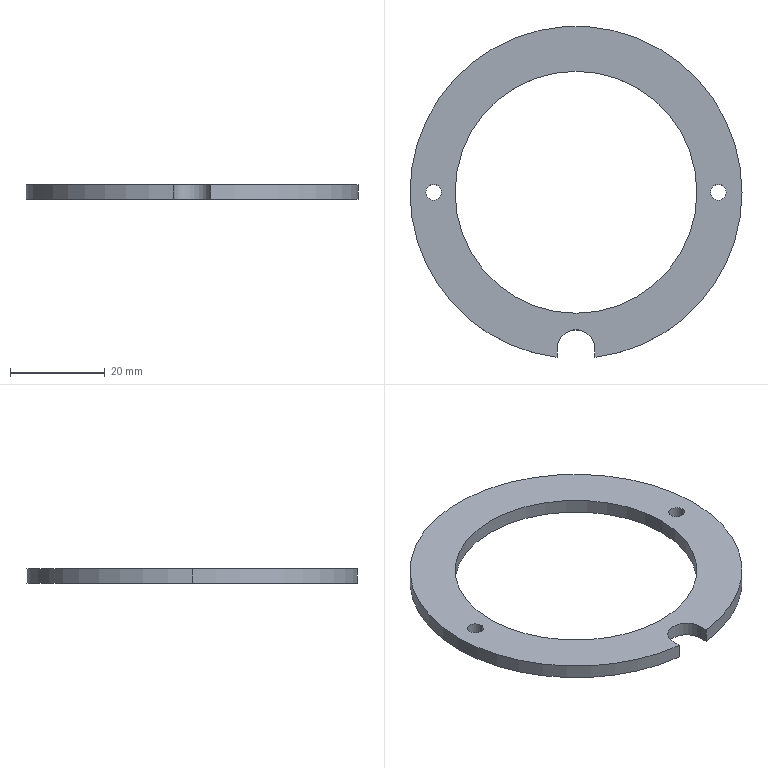Part | SolidWorks | features ICE 4, Extrusion 1, HoleWzd 1 | 1 solid | 14 faces | box 70 x 69.771 x 3 mm | volume 5244 mm3 | cylinder 10 | plane 4 | commonest cylinder face diameters 3.3 x4 70 x3 51 x2 8 x1
STEP:
#1=CARTESIAN_POINT('',(28.35,0.,0.));
#2=VERTEX_POINT('',#1);
#3=CARTESIAN_POINT('',(31.65,0.,0.));
#4=VERTEX_POINT('',#3);
#5=CARTESIAN_POINT('',(30.,0.,0.));
#6=DIRECTION('',(0.,0.,1.));
#7=DIRECTION('',(1.,0.,0.));
#8=AXIS2_PLACEMENT_3D('',#5,#6,#7);
#9=CIRCLE('',#8,1.65);
#10=EDGE_CURVE('',#2,#4,#9,.T.);
#11=ORIENTED_EDGE('',*,*,#10,.F.);
#12=CARTESIAN_POINT('',(28.35,0.,3.));
#13=VERTEX_POINT('',#12);
#14=CARTESIAN_POINT('',(28.35,0.,0.));
#15=DIRECTION('',(0.,0.,1.));
#16=VECTOR('',#15,1000.);
#17=LINE('',#14,#16);
#18=EDGE_CURVE('',#2,#13,#17,.T.);
#19=ORIENTED_EDGE('',*,*,#18,.T.);
#20=CARTESIAN_POINT('',(31.65,0.,3.));
#21=VERTEX_POINT('',#20);
#22=CARTESIAN_POINT('',(30.,0.,3.));
#23=DIRECTION('',(0.,0.,1.));
#24=DIRECTION('',(1.,0.,0.));
#25=AXIS2_PLACEMENT_3D('',#22,#23,#24);
#26=CIRCLE('',#25,1.65);
#27=EDGE_CURVE('',#13,#21,#26,.T.);
#28=ORIENTED_EDGE('',*,*,#27,.T.);
#29=CARTESIAN_POINT('',(31.65,0.,0.));
#30=DIRECTION('',(0.,0.,1.));
#31=VECTOR('',#30,1000.);
#32=LINE('',#29,#31);
#33=EDGE_CURVE('',#4,#21,#32,.T.);
#34=ORIENTED_EDGE('',*,*,#33,.F.);
#35=EDGE_LOOP('',(#11,#19,#28,#34));
#36=FACE_OUTER_BOUND('',#35,.T.);
#37=CARTESIAN_POINT('',(30.,0.,0.));
#38=DIRECTION('',(0.,0.,1.));
#39=DIRECTION('',(1.,0.,0.));
#40=AXIS2_PLACEMENT_3D('',#37,#38,#39);
#41=CYLINDRICAL_SURFACE('',#40,1.65);
#42=ADVANCED_FACE('',(#36),#41,.F.);
#43=CARTESIAN_POINT('',(-31.65,0.,0.));
#44=VERTEX_POINT('',#43);
#45=CARTESIAN_POINT('',(-28.35,0.,0.));
#46=VERTEX_POINT('',#45);
#47=CARTESIAN_POINT('',(-30.,0.,0.));
#48=DIRECTION('',(0.,0.,1.));
#49=DIRECTION('',(-1.,0.,0.));
#50=AXIS2_PLACEMENT_3D('',#47,#48,#49);
#51=CIRCLE('',#50,1.65);
#52=EDGE_CURVE('',#44,#46,#51,.T.);
#53=ORIENTED_EDGE('',*,*,#52,.F.);
#54=CARTESIAN_POINT('',(-31.65,0.,3.));
#55=VERTEX_POINT('',#54);
#56=CARTESIAN_POINT('',(-31.65,0.,0.));
#57=DIRECTION('',(0.,0.,1.));
#58=VECTOR('',#57,1000.);
#59=LINE('',#56,#58);
#60=EDGE_CURVE('',#44,#55,#59,.T.);
#61=ORIENTED_EDGE('',*,*,#60,.T.);
#62=CARTESIAN_POINT('',(-28.35,0.,3.));
#63=VERTEX_POINT('',#62);
#64=CARTESIAN_POINT('',(-30.,0.,3.));
#65=DIRECTION('',(0.,0.,1.));
#66=DIRECTION('',(-1.,0.,0.));
#67=AXIS2_PLACEMENT_3D('',#64,#65,#66);
#68=CIRCLE('',#67,1.65);
#69=EDGE_CURVE('',#55,#63,#68,.T.);
#70=ORIENTED_EDGE('',*,*,#69,.T.);
#71=CARTESIAN_POINT('',(-28.35,0.,0.));
#72=DIRECTION('',(0.,0.,1.));
#73=VECTOR('',#72,1000.);
#74=LINE('',#71,#73);
#75=EDGE_CURVE('',#46,#63,#74,.T.);
#76=ORIENTED_EDGE('',*,*,#75,.F.);
#77=EDGE_LOOP('',(#53,#61,#70,#76));
#78=FACE_OUTER_BOUND('',#77,.T.);
#79=CARTESIAN_POINT('',(-30.,0.,0.));
#80=DIRECTION('',(0.,0.,1.));
#81=DIRECTION('',(1.,0.,0.));
#82=AXIS2_PLACEMENT_3D('',#79,#80,#81);
#83=CYLINDRICAL_SURFACE('',#82,1.65);
#84=ADVANCED_FACE('',(#78),#83,.F.);
#85=CARTESIAN_POINT('',(-25.5,0.,3.));
#86=VERTEX_POINT('',#85);
#87=CARTESIAN_POINT('',(25.5,0.,3.));
#88=VERTEX_POINT('',#87);
#89=CARTESIAN_POINT('',(0.,0.,3.));
#90=DIRECTION('',(0.,0.,1.));
#91=DIRECTION('',(1.,0.,0.));
#92=AXIS2_PLACEMENT_3D('',#89,#90,#91);
#93=CIRCLE('',#92,25.5);
#94=EDGE_CURVE('',#86,#88,#93,.T.);
#95=ORIENTED_EDGE('',*,*,#94,.T.);
#96=CARTESIAN_POINT('',(25.5,0.,0.));
#97=VERTEX_POINT('',#96);
#98=CARTESIAN_POINT('',(25.5,0.,3.));
#99=DIRECTION('',(0.,0.,-1.));
#100=VECTOR('',#99,1000.);
#101=LINE('',#98,#100);
#102=EDGE_CURVE('',#88,#97,#101,.T.);
#103=ORIENTED_EDGE('',*,*,#102,.T.);
#104=CARTESIAN_POINT('',(-25.5,0.,0.));
#105=VERTEX_POINT('',#104);
#106=CARTESIAN_POINT('',(0.,0.,0.));
#107=DIRECTION('',(0.,0.,1.));
#108=DIRECTION('',(1.,0.,0.));
#109=AXIS2_PLACEMENT_3D('',#106,#107,#108);
#110=CIRCLE('',#109,25.5);
#111=EDGE_CURVE('',#105,#97,#110,.T.);
#112=ORIENTED_EDGE('',*,*,#111,.F.);
#113=CARTESIAN_POINT('',(-25.5,0.,3.));
#114=DIRECTION('',(0.,0.,-1.));
#115=VECTOR('',#114,1000.);
#116=LINE('',#113,#115);
#117=EDGE_CURVE('',#86,#105,#116,.T.);
#118=ORIENTED_EDGE('',*,*,#117,.F.);
#119=EDGE_LOOP('',(#95,#103,#112,#118));
#120=FACE_OUTER_BOUND('',#119,.T.);
#121=CARTESIAN_POINT('',(0.,0.,3.));
#122=DIRECTION('',(0.,0.,-1.));
#123=DIRECTION('',(-1.,0.,0.));
#124=AXIS2_PLACEMENT_3D('',#121,#122,#123);
#125=CYLINDRICAL_SURFACE('',#124,25.5);
#126=ADVANCED_FACE('',(#120),#125,.F.);
#127=CARTESIAN_POINT('',(35.,0.,3.));
#128=VERTEX_POINT('',#127);
#129=CARTESIAN_POINT('',(-35.,0.,3.));
#130=VERTEX_POINT('',#129);
#131=CARTESIAN_POINT('',(0.,0.,3.));
#132=DIRECTION('',(0.,0.,1.));
#133=DIRECTION('',(1.,0.,0.));
#134=AXIS2_PLACEMENT_3D('',#131,#132,#133);
#135=CIRCLE('',#134,35.);
#136=EDGE_CURVE('',#128,#130,#135,.T.);
#137=ORIENTED_EDGE('',*,*,#136,.F.);
#138=CARTESIAN_POINT('',(35.,0.,0.));
#139=VERTEX_POINT('',#138);
#140=CARTESIAN_POINT('',(35.,0.,3.));
#141=DIRECTION('',(0.,0.,-1.));
#142=VECTOR('',#141,1000.);
#143=LINE('',#140,#142);
#144=EDGE_CURVE('',#128,#139,#143,.T.);
#145=ORIENTED_EDGE('',*,*,#144,.T.);
#146=CARTESIAN_POINT('',(-35.,0.,0.));
#147=VERTEX_POINT('',#146);
#148=CARTESIAN_POINT('',(0.,0.,0.));
#149=DIRECTION('',(0.,0.,1.));
#150=DIRECTION('',(1.,0.,0.));
#151=AXIS2_PLACEMENT_3D('',#148,#149,#150);
#152=CIRCLE('',#151,35.);
#153=EDGE_CURVE('',#139,#147,#152,.T.);
#154=ORIENTED_EDGE('',*,*,#153,.T.);
#155=CARTESIAN_POINT('',(-35.,0.,3.));
#156=DIRECTION('',(0.,0.,-1.));
#157=VECTOR('',#156,1000.);
#158=LINE('',#155,#157);
#159=EDGE_CURVE('',#130,#147,#158,.T.);
#160=ORIENTED_EDGE('',*,*,#159,.F.);
#161=EDGE_LOOP('',(#137,#145,#154,#160));
#162=FACE_OUTER_BOUND('',#161,.T.);
#163=CARTESIAN_POINT('',(0.,0.,3.));
#164=DIRECTION('',(0.,0.,-1.));
#165=DIRECTION('',(-1.,0.,0.));
#166=AXIS2_PLACEMENT_3D('',#163,#164,#165);
#167=CYLINDRICAL_SURFACE('',#166,35.);
#168=ADVANCED_FACE('',(#162),#167,.T.);
#169=CARTESIAN_POINT('',(-4.,-34.771,3.));
#170=VERTEX_POINT('',#169);
#171=CARTESIAN_POINT('',(0.,0.,3.));
#172=DIRECTION('',(0.,0.,1.));
#173=DIRECTION('',(1.,0.,0.));
#174=AXIS2_PLACEMENT_3D('',#171,#172,#173);
#175=CIRCLE('',#174,35.);
#176=EDGE_CURVE('',#130,#170,#175,.T.);
#177=ORIENTED_EDGE('',*,*,#176,.F.);
#178=ORIENTED_EDGE('',*,*,#159,.T.);
#179=CARTESIAN_POINT('',(-4.,-34.771,0.));
#180=VERTEX_POINT('',#179);
#181=CARTESIAN_POINT('',(0.,0.,0.));
#182=DIRECTION('',(0.,0.,1.));
#183=DIRECTION('',(1.,0.,0.));
#184=AXIS2_PLACEMENT_3D('',#181,#182,#183);
#185=CIRCLE('',#184,35.);
#186=EDGE_CURVE('',#147,#180,#185,.T.);
#187=ORIENTED_EDGE('',*,*,#186,.T.);
#188=CARTESIAN_POINT('',(-4.,-34.771,3.));
#189=DIRECTION('',(0.,0.,1.));
#190=VECTOR('',#189,1000.);
#191=LINE('',#188,#190);
#192=EDGE_CURVE('',#180,#170,#191,.T.);
#193=ORIENTED_EDGE('',*,*,#192,.T.);
#194=EDGE_LOOP('',(#177,#178,#187,#193));
#195=FACE_OUTER_BOUND('',#194,.T.);
#196=CARTESIAN_POINT('',(0.,0.,3.));
#197=DIRECTION('',(0.,0.,-1.));
#198=DIRECTION('',(-1.,0.,0.));
#199=AXIS2_PLACEMENT_3D('',#196,#197,#198);
#200=CYLINDRICAL_SURFACE('',#199,35.);
#201=ADVANCED_FACE('',(#195),#200,.T.);
#202=CARTESIAN_POINT('',(30.,0.,3.));
#203=DIRECTION('',(0.,0.,1.));
#204=DIRECTION('',(1.,0.,0.));
#205=AXIS2_PLACEMENT_3D('',#202,#203,#204);
#206=CIRCLE('',#205,1.65);
#207=EDGE_CURVE('',#21,#13,#206,.T.);
#208=ORIENTED_EDGE('',*,*,#207,.F.);
#209=ORIENTED_EDGE('',*,*,#27,.F.);
#210=EDGE_LOOP('',(#208,#209));
#211=FACE_BOUND('',#210,.T.);
#212=CARTESIAN_POINT('',(-30.,0.,3.));
#213=DIRECTION('',(0.,0.,1.));
#214=DIRECTION('',(-1.,0.,0.));
#215=AXIS2_PLACEMENT_3D('',#212,#213,#214);
#216=CIRCLE('',#215,1.65);
#217=EDGE_CURVE('',#63,#55,#216,.T.);
#218=ORIENTED_EDGE('',*,*,#217,.F.);
#219=ORIENTED_EDGE('',*,*,#69,.F.);
#220=EDGE_LOOP('',(#218,#219));
#221=FACE_BOUND('',#220,.T.);
#222=CARTESIAN_POINT('',(4.,-34.771,3.));
#223=VERTEX_POINT('',#222);
#224=CARTESIAN_POINT('',(4.,-33.,3.));
#225=VERTEX_POINT('',#224);
#226=CARTESIAN_POINT('',(4.,-33.,3.));
#227=DIRECTION('',(0.,1.,0.));
#228=VECTOR('',#227,1000.);
#229=LINE('',#226,#228);
#230=EDGE_CURVE('',#223,#225,#229,.T.);
#231=ORIENTED_EDGE('',*,*,#230,.F.);
#232=CARTESIAN_POINT('',(0.,0.,3.));
#233=DIRECTION('',(0.,0.,1.));
#234=DIRECTION('',(1.,0.,0.));
#235=AXIS2_PLACEMENT_3D('',#232,#233,#234);
#236=CIRCLE('',#235,35.);
#237=EDGE_CURVE('',#223,#128,#236,.T.);
#238=ORIENTED_EDGE('',*,*,#237,.T.);
#239=ORIENTED_EDGE('',*,*,#136,.T.);
#240=ORIENTED_EDGE('',*,*,#176,.T.);
#241=CARTESIAN_POINT('',(-4.,-33.,3.));
#242=VERTEX_POINT('',#241);
#243=CARTESIAN_POINT('',(-4.,-33.,3.));
#244=DIRECTION('',(0.,-1.,0.));
#245=VECTOR('',#244,1000.);
#246=LINE('',#243,#245);
#247=EDGE_CURVE('',#242,#170,#246,.T.);
#248=ORIENTED_EDGE('',*,*,#247,.F.);
#249=CARTESIAN_POINT('',(0.,-33.,3.));
#250=DIRECTION('',(0.,0.,1.));
#251=DIRECTION('',(1.,0.,0.));
#252=AXIS2_PLACEMENT_3D('',#249,#250,#251);
#253=CIRCLE('',#252,4.);
#254=EDGE_CURVE('',#225,#242,#253,.T.);
#255=ORIENTED_EDGE('',*,*,#254,.F.);
#256=EDGE_LOOP('',(#231,#238,#239,#240,#248,#255));
#257=FACE_OUTER_BOUND('',#256,.T.);
#258=ORIENTED_EDGE('',*,*,#94,.F.);
#259=CARTESIAN_POINT('',(0.,0.,3.));
#260=DIRECTION('',(0.,0.,1.));
#261=DIRECTION('',(1.,0.,0.));
#262=AXIS2_PLACEMENT_3D('',#259,#260,#261);
#263=CIRCLE('',#262,25.5);
#264=EDGE_CURVE('',#88,#86,#263,.T.);
#265=ORIENTED_EDGE('',*,*,#264,.F.);
#266=EDGE_LOOP('',(#258,#265));
#267=FACE_BOUND('',#266,.T.);
#268=CARTESIAN_POINT('',(0.,0.,3.));
#269=DIRECTION('',(0.,0.,1.));
#270=DIRECTION('',(1.,0.,0.));
#271=AXIS2_PLACEMENT_3D('',#268,#269,#270);
#272=PLANE('',#271);
#273=ADVANCED_FACE('',(#211,#221,#257,#267),#272,.T.);
#274=CARTESIAN_POINT('',(30.,0.,0.));
#275=DIRECTION('',(0.,0.,1.));
#276=DIRECTION('',(1.,0.,0.));
#277=AXIS2_PLACEMENT_3D('',#274,#275,#276);
#278=CIRCLE('',#277,1.65);
#279=EDGE_CURVE('',#4,#2,#278,.T.);
#280=ORIENTED_EDGE('',*,*,#279,.T.);
#281=ORIENTED_EDGE('',*,*,#10,.T.);
#282=EDGE_LOOP('',(#280,#281));
#283=FACE_BOUND('',#282,.T.);
#284=CARTESIAN_POINT('',(-30.,0.,0.));
#285=DIRECTION('',(0.,0.,1.));
#286=DIRECTION('',(-1.,0.,0.));
#287=AXIS2_PLACEMENT_3D('',#284,#285,#286);
#288=CIRCLE('',#287,1.65);
#289=EDGE_CURVE('',#46,#44,#288,.T.);
#290=ORIENTED_EDGE('',*,*,#289,.T.);
#291=ORIENTED_EDGE('',*,*,#52,.T.);
#292=EDGE_LOOP('',(#290,#291));
#293=FACE_BOUND('',#292,.T.);
#294=CARTESIAN_POINT('',(4.,-34.771,0.));
#295=VERTEX_POINT('',#294);
#296=CARTESIAN_POINT('',(0.,0.,0.));
#297=DIRECTION('',(0.,0.,1.));
#298=DIRECTION('',(1.,0.,0.));
#299=AXIS2_PLACEMENT_3D('',#296,#297,#298);
#300=CIRCLE('',#299,35.);
#301=EDGE_CURVE('',#295,#139,#300,.T.);
#302=ORIENTED_EDGE('',*,*,#301,.F.);
#303=CARTESIAN_POINT('',(4.,-33.,0.));
#304=VERTEX_POINT('',#303);
#305=CARTESIAN_POINT('',(4.,-33.,0.));
#306=DIRECTION('',(0.,1.,0.));
#307=VECTOR('',#306,1000.);
#308=LINE('',#305,#307);
#309=EDGE_CURVE('',#295,#304,#308,.T.);
#310=ORIENTED_EDGE('',*,*,#309,.T.);
#311=CARTESIAN_POINT('',(-4.,-33.,0.));
#312=VERTEX_POINT('',#311);
#313=CARTESIAN_POINT('',(0.,-33.,0.));
#314=DIRECTION('',(0.,0.,-1.));
#315=DIRECTION('',(-1.,0.,0.));
#316=AXIS2_PLACEMENT_3D('',#313,#314,#315);
#317=CIRCLE('',#316,4.);
#318=EDGE_CURVE('',#312,#304,#317,.T.);
#319=ORIENTED_EDGE('',*,*,#318,.F.);
#320=CARTESIAN_POINT('',(-4.,-33.,0.));
#321=DIRECTION('',(0.,-1.,0.));
#322=VECTOR('',#321,1000.);
#323=LINE('',#320,#322);
#324=EDGE_CURVE('',#312,#180,#323,.T.);
#325=ORIENTED_EDGE('',*,*,#324,.T.);
#326=ORIENTED_EDGE('',*,*,#186,.F.);
#327=ORIENTED_EDGE('',*,*,#153,.F.);
#328=EDGE_LOOP('',(#302,#310,#319,#325,#326,#327));
#329=FACE_OUTER_BOUND('',#328,.T.);
#330=ORIENTED_EDGE('',*,*,#111,.T.);
#331=CARTESIAN_POINT('',(0.,0.,0.));
#332=DIRECTION('',(0.,0.,1.));
#333=DIRECTION('',(1.,0.,0.));
#334=AXIS2_PLACEMENT_3D('',#331,#332,#333);
#335=CIRCLE('',#334,25.5);
#336=EDGE_CURVE('',#97,#105,#335,.T.);
#337=ORIENTED_EDGE('',*,*,#336,.T.);
#338=EDGE_LOOP('',(#330,#337));
#339=FACE_BOUND('',#338,.T.);
#340=CARTESIAN_POINT('',(0.,0.,0.));
#341=DIRECTION('',(0.,0.,1.));
#342=DIRECTION('',(1.,0.,0.));
#343=AXIS2_PLACEMENT_3D('',#340,#341,#342);
#344=PLANE('',#343);
#345=ADVANCED_FACE('',(#283,#293,#329,#339),#344,.F.);
#346=ORIENTED_EDGE('',*,*,#144,.F.);
#347=ORIENTED_EDGE('',*,*,#237,.F.);
#348=CARTESIAN_POINT('',(4.,-34.771,3.));
#349=DIRECTION('',(0.,0.,-1.));
#350=VECTOR('',#349,1000.);
#351=LINE('',#348,#350);
#352=EDGE_CURVE('',#223,#295,#351,.T.);
#353=ORIENTED_EDGE('',*,*,#352,.T.);
#354=ORIENTED_EDGE('',*,*,#301,.T.);
#355=EDGE_LOOP('',(#346,#347,#353,#354));
#356=FACE_OUTER_BOUND('',#355,.T.);
#357=CARTESIAN_POINT('',(0.,0.,3.));
#358=DIRECTION('',(0.,0.,-1.));
#359=DIRECTION('',(-1.,0.,0.));
#360=AXIS2_PLACEMENT_3D('',#357,#358,#359);
#361=CYLINDRICAL_SURFACE('',#360,35.);
#362=ADVANCED_FACE('',(#356),#361,.T.);
#363=ORIENTED_EDGE('',*,*,#102,.F.);
#364=ORIENTED_EDGE('',*,*,#264,.T.);
#365=ORIENTED_EDGE('',*,*,#117,.T.);
#366=ORIENTED_EDGE('',*,*,#336,.F.);
#367=EDGE_LOOP('',(#363,#364,#365,#366));
#368=FACE_OUTER_BOUND('',#367,.T.);
#369=CARTESIAN_POINT('',(0.,0.,3.));
#370=DIRECTION('',(0.,0.,-1.));
#371=DIRECTION('',(-1.,0.,0.));
#372=AXIS2_PLACEMENT_3D('',#369,#370,#371);
#373=CYLINDRICAL_SURFACE('',#372,25.5);
#374=ADVANCED_FACE('',(#368),#373,.F.);
#375=ORIENTED_EDGE('',*,*,#318,.T.);
#376=CARTESIAN_POINT('',(4.,-33.,0.));
#377=DIRECTION('',(0.,0.,1.));
#378=VECTOR('',#377,1000.);
#379=LINE('',#376,#378);
#380=EDGE_CURVE('',#304,#225,#379,.T.);
#381=ORIENTED_EDGE('',*,*,#380,.T.);
#382=ORIENTED_EDGE('',*,*,#254,.T.);
#383=CARTESIAN_POINT('',(-4.,-33.,0.));
#384=DIRECTION('',(0.,0.,1.));
#385=VECTOR('',#384,1000.);
#386=LINE('',#383,#385);
#387=EDGE_CURVE('',#312,#242,#386,.T.);
#388=ORIENTED_EDGE('',*,*,#387,.F.);
#389=EDGE_LOOP('',(#375,#381,#382,#388));
#390=FACE_OUTER_BOUND('',#389,.T.);
#391=CARTESIAN_POINT('',(0.,-33.,5.));
#392=DIRECTION('',(0.,0.,-1.));
#393=DIRECTION('',(-1.,0.,0.));
#394=AXIS2_PLACEMENT_3D('',#391,#392,#393);
#395=CYLINDRICAL_SURFACE('',#394,4.);
#396=ADVANCED_FACE('',(#390),#395,.F.);
#397=ORIENTED_EDGE('',*,*,#324,.F.);
#398=ORIENTED_EDGE('',*,*,#387,.T.);
#399=ORIENTED_EDGE('',*,*,#247,.T.);
#400=ORIENTED_EDGE('',*,*,#192,.F.);
#401=EDGE_LOOP('',(#397,#398,#399,#400));
#402=FACE_OUTER_BOUND('',#401,.T.);
#403=CARTESIAN_POINT('',(-4.,-33.,0.));
#404=DIRECTION('',(-1.,0.,0.));
#405=DIRECTION('',(0.,-1.,0.));
#406=AXIS2_PLACEMENT_3D('',#403,#404,#405);
#407=PLANE('',#406);
#408=ADVANCED_FACE('',(#402),#407,.F.);
#409=ORIENTED_EDGE('',*,*,#230,.T.);
#410=ORIENTED_EDGE('',*,*,#380,.F.);
#411=ORIENTED_EDGE('',*,*,#309,.F.);
#412=ORIENTED_EDGE('',*,*,#352,.F.);
#413=EDGE_LOOP('',(#409,#410,#411,#412));
#414=FACE_OUTER_BOUND('',#413,.T.);
#415=CARTESIAN_POINT('',(4.,-33.,0.));
#416=DIRECTION('',(1.,0.,0.));
#417=DIRECTION('',(0.,1.,0.));
#418=AXIS2_PLACEMENT_3D('',#415,#416,#417);
#419=PLANE('',#418);
#420=ADVANCED_FACE('',(#414),#419,.F.);
#421=ORIENTED_EDGE('',*,*,#60,.F.);
#422=ORIENTED_EDGE('',*,*,#289,.F.);
#423=ORIENTED_EDGE('',*,*,#75,.T.);
#424=ORIENTED_EDGE('',*,*,#217,.T.);
#425=EDGE_LOOP('',(#421,#422,#423,#424));
#426=FACE_OUTER_BOUND('',#425,.T.);
#427=CARTESIAN_POINT('',(-30.,0.,0.));
#428=DIRECTION('',(0.,0.,1.));
#429=DIRECTION('',(1.,0.,0.));
#430=AXIS2_PLACEMENT_3D('',#427,#428,#429);
#431=CYLINDRICAL_SURFACE('',#430,1.65);
#432=ADVANCED_FACE('',(#426),#431,.F.);
#433=ORIENTED_EDGE('',*,*,#18,.F.);
#434=ORIENTED_EDGE('',*,*,#279,.F.);
#435=ORIENTED_EDGE('',*,*,#33,.T.);
#436=ORIENTED_EDGE('',*,*,#207,.T.);
#437=EDGE_LOOP('',(#433,#434,#435,#436));
#438=FACE_OUTER_BOUND('',#437,.T.);
#439=CARTESIAN_POINT('',(30.,0.,0.));
#440=DIRECTION('',(0.,0.,1.));
#441=DIRECTION('',(1.,0.,0.));
#442=AXIS2_PLACEMENT_3D('',#439,#440,#441);
#443=CYLINDRICAL_SURFACE('',#442,1.65);
#444=ADVANCED_FACE('',(#438),#443,.F.);
#445=CLOSED_SHELL('',(#42,#84,#126,#168,#201,#273,#345,#362,#374,#396,#408,#420,#432,#444));
#446=MANIFOLD_SOLID_BREP('',#445);
#447=CARTESIAN_POINT('',(0.,0.,0.));
#448=DIRECTION('',(0.,0.,1.));
#449=DIRECTION('',(1.,0.,0.));
#450=AXIS2_PLACEMENT_3D('',#447,#448,#449);
#451=(LENGTH_UNIT()NAMED_UNIT(*)SI_UNIT(.MILLI.,.METRE.));
#452=UNCERTAINTY_MEASURE_WITH_UNIT(LENGTH_MEASURE(0.00001),#451,'','');
#453=(NAMED_UNIT(*)PLANE_ANGLE_UNIT()SI_UNIT($,.RADIAN.));
#454=(NAMED_UNIT(*)SI_UNIT($,.STERADIAN.)SOLID_ANGLE_UNIT());
#455=(GEOMETRIC_REPRESENTATION_CONTEXT(3)GLOBAL_UNCERTAINTY_ASSIGNED_CONTEXT((#452))GLOBAL_UNIT_ASSIGNED_CONTEXT((#451,#453,#454))REPRESENTATION_CONTEXT('',''));
#456=ADVANCED_BREP_SHAPE_REPRESENTATION('',(#446,#450),#455);